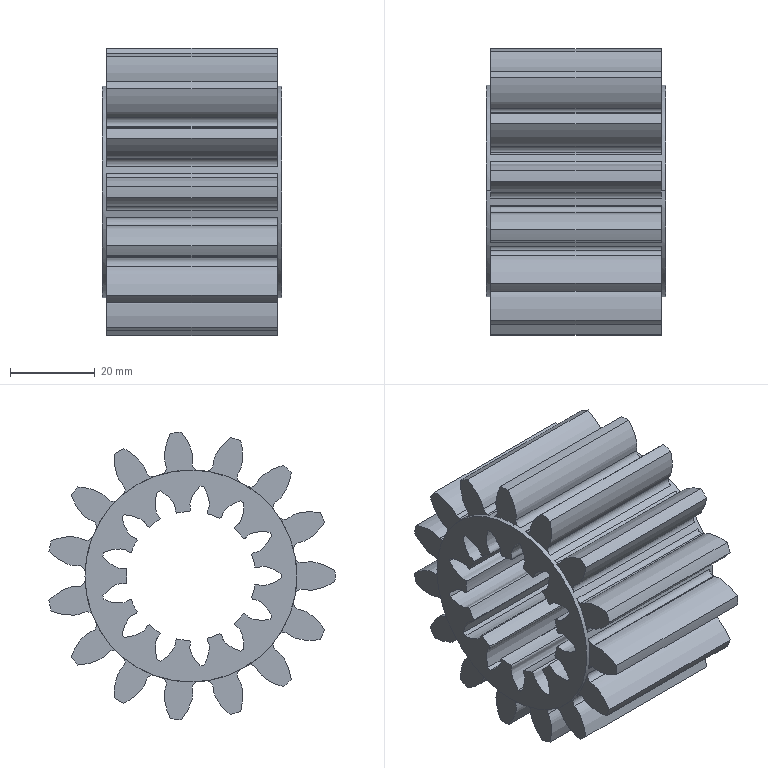Part | NX | features BREP 1 | 1 solid | 168 faces | box 42.3 x 67.504 x 67.851 mm | volume 71690 mm3 | cylinder 80 | spline 56 | plane 32 | commonest cylinder face diameters 3.04 x37 68 x15 30.411 x13 42.625 x13 50 x2